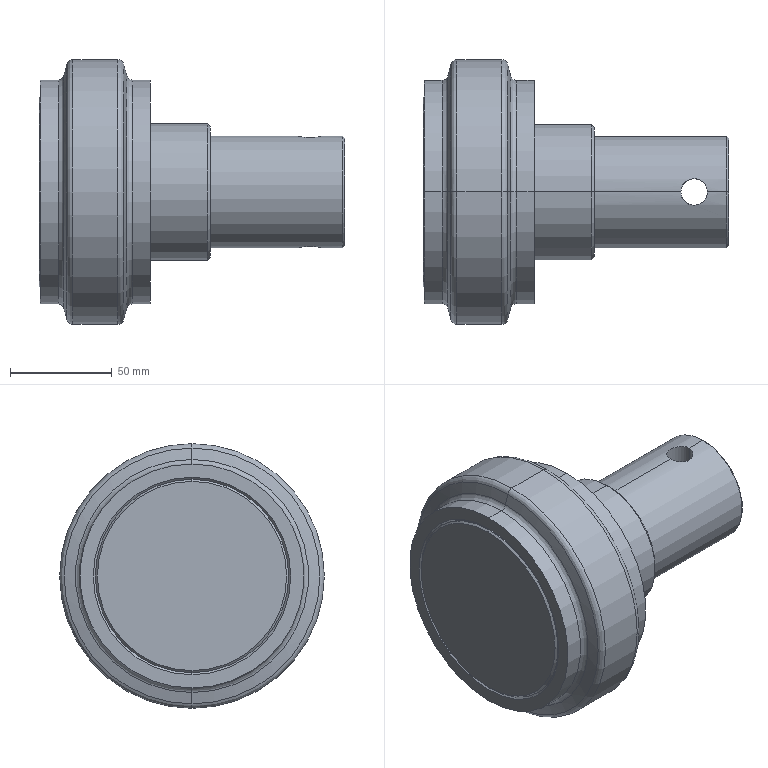Part | SolidWorks | 5 solids | 659 faces | box 150 x 130 x 130 mm | volume 834716 mm3 | cylinder 340 | plane 253 | torus 34 | cone 32 | commonest cylinder face diameters 8.02 x174 69.5 x60 85.5 x60 95 x10 81.225 x8 60 x6